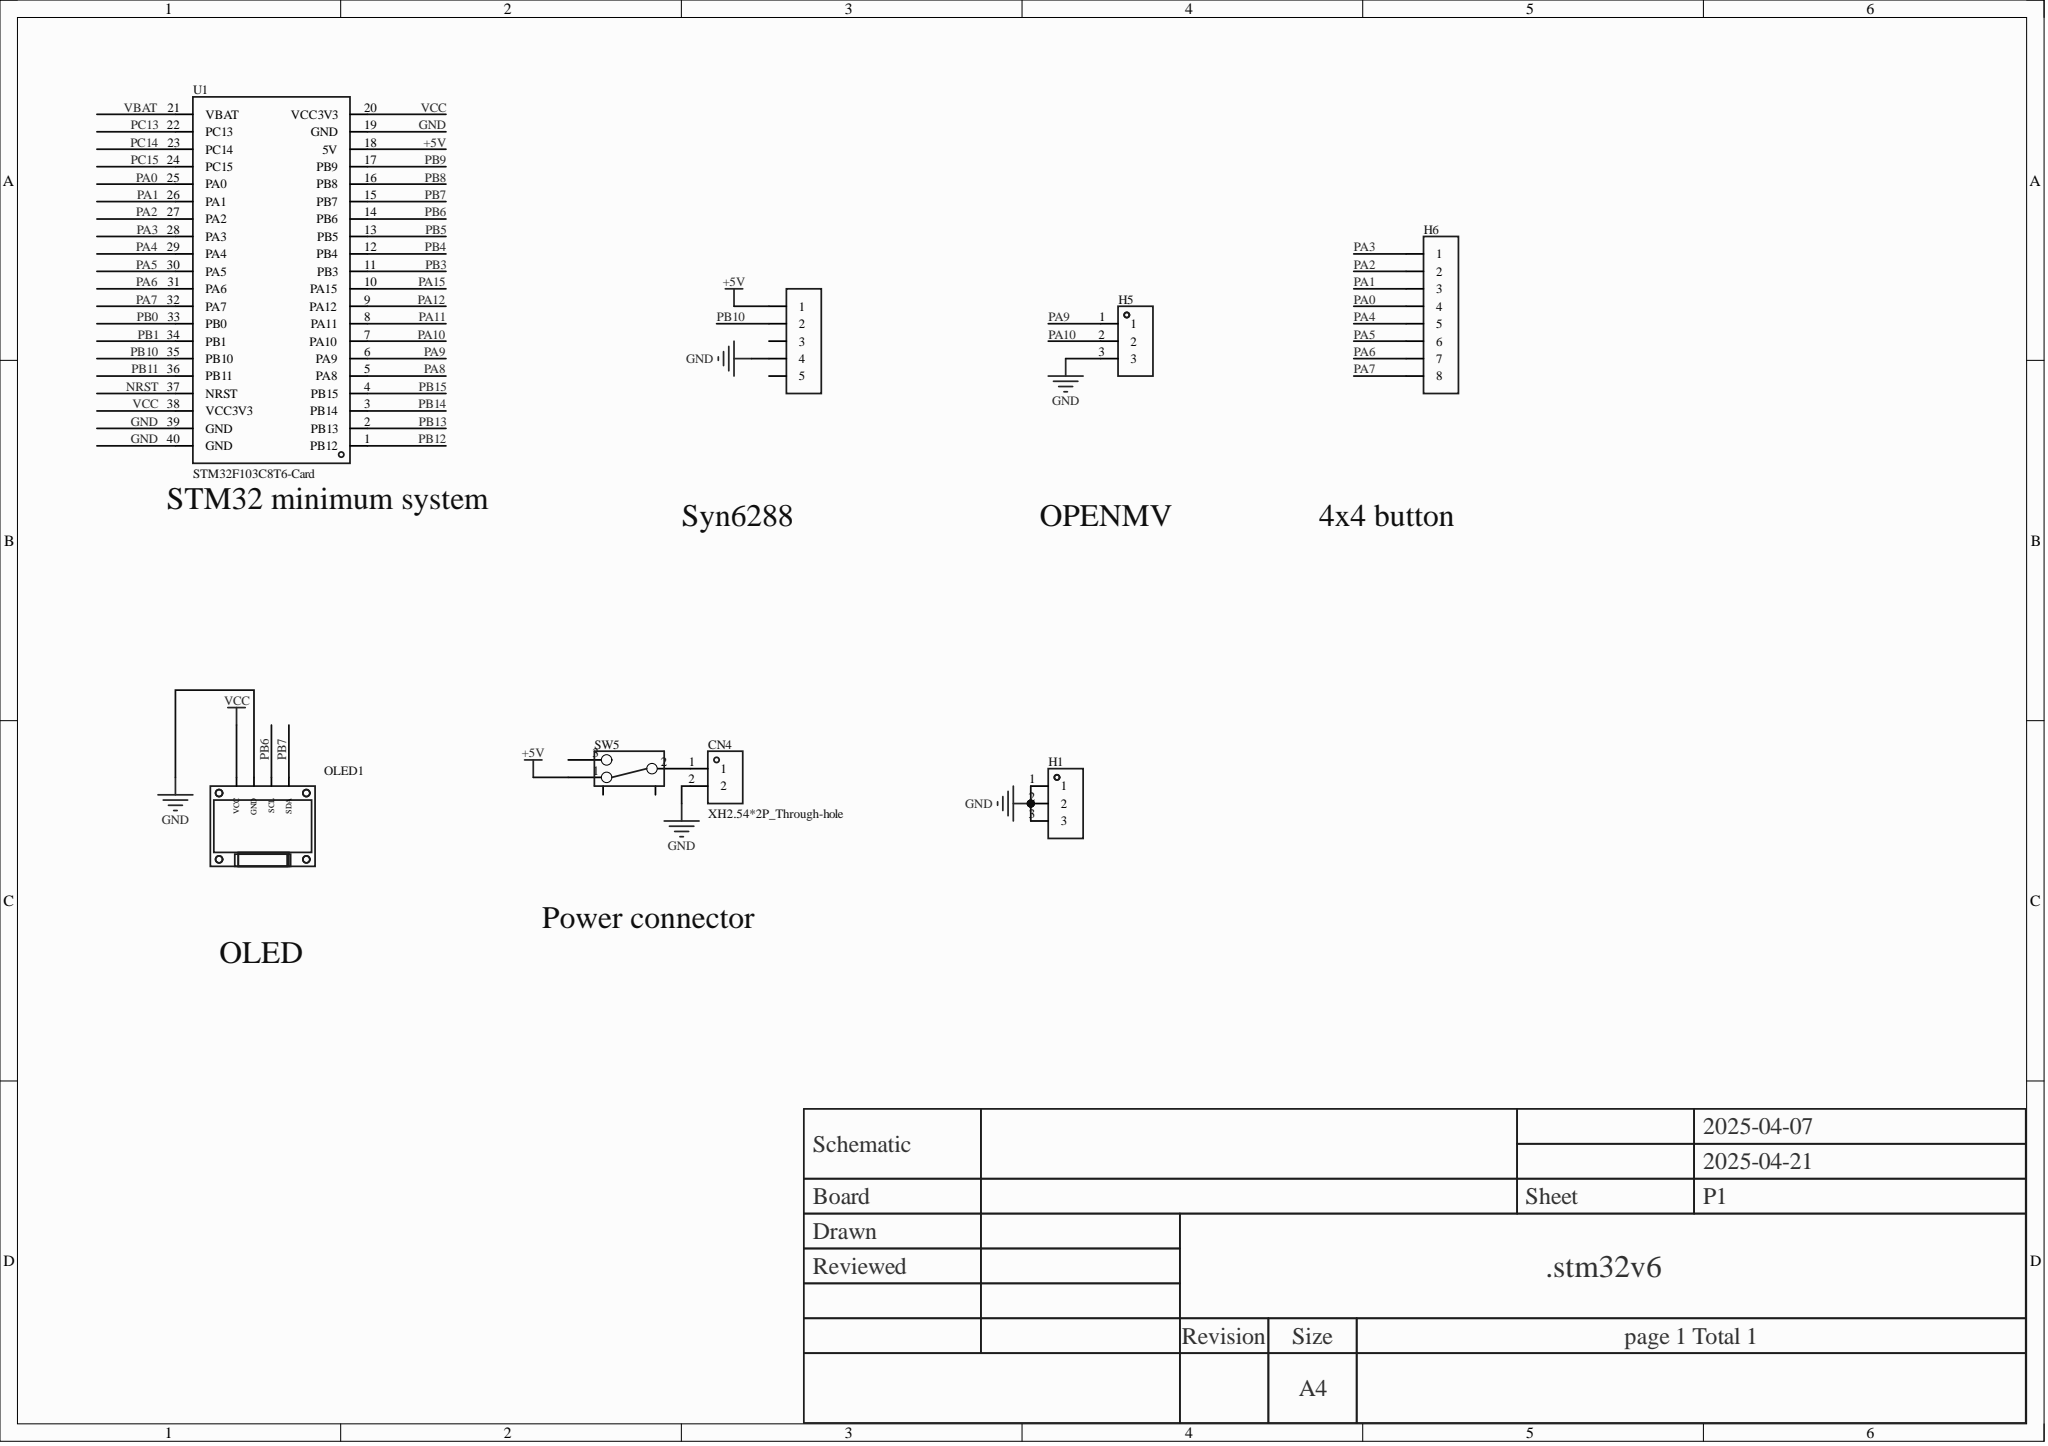Circuit board | Altium Designer | 8 parts | 17 nets
Bill of materials:
Comment,Description,Designator,Footprint,LibRef,Quantity
"XH2.54*2P_Through-hole","","CN4","CONN-TH_2P-P2.50-XH2.54-2P","XH2.54*2P_直插","1"
"","","H1, H5","HDR-TH_3P-P2.54-V-M","HDR-M_2.54_1x3P","2"
"","","H6","HDR-TH_8P-P2.54-V-F-1","HDR-F_2.54_1x8P","1"
"","","OLED1","0.96OLED_4P","0.96OLED模块_4P","1"
"","","SW5","拨动开关","拨动开关_正","1"
"STM32F103C8T6-Card","","U1","CONN-TH_L53.3-W22.9_STM32F103C8T6-CARD","STM32F103C8T6-Card","1"
"","","插槽出版子","HDR-TH_5P-P2.54-V-F","HDR-F_2.54_1x5P","1"
Netlist (Protel format):
[
CN4
CONN-TH_2P-P2.50-XH2.54-2P
XH2.54*2P_Through-hole



]
[
H1
HDR-TH_3P-P2.54-V-M




]
[
H5
HDR-TH_3P-P2.54-V-M




]
[
H6
HDR-TH_8P-P2.54-V-F-1




]
[
OLED1
0.96OLED_4P




]
[
SW5
拨动开关




]
[
U1
CONN-TH_L53.3-W22.9_STM32F103C8T6-CARD
STM32F103C8T6-Card



]
[
插槽出版子
HDR-TH_5P-P2.54-V-F




]
(
VCC
OLED1-1
U1-20
U1-38
)
(
PB10
U1-35
插槽出版子-2
)
(
PB7
OLED1-4
U1-15
)
(
PB6
OLED1-3
U1-14
)
(
PA10
H5-2
U1-7
)
(
PA9
H5-1
U1-6
)
(
PA7
H6-8
U1-32
)
(
PA6
H6-7
U1-31
)
(
PA5
H6-6
U1-30
)
(
PA4
H6-5
U1-29
)
(
PA3
H6-1
U1-28
)
(
PA2
H6-2
U1-27
)
(
PA1
H6-3
U1-26
)
(
PA0
H6-4
U1-25
)
(
NetCN4_1
CN4-1
SW5-2
)
(
GND
CN4-2
H1-1
H1-2
H1-3
H5-3
OLED1-2
U1-19
U1-39
U1-40
插槽出版子-4
)
(
+5V
SW5-1
U1-18
插槽出版子-1
)